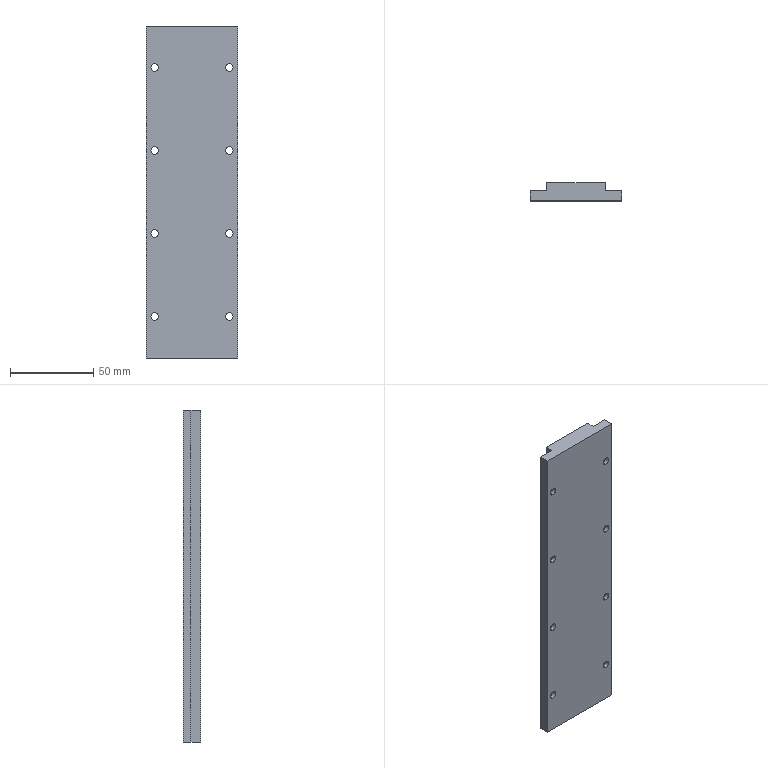Part | SolidWorks | features BaseBody 1 | 1 solid | 50 faces | box 55 x 10.7 x 200 mm | volume 97550 mm3 | cylinder 32 | plane 18 | commonest cylinder face diameters 4.5 x16 8 x16
STEP:
#1=CARTESIAN_POINT('',(5.,0.,27.25));
#2=VERTEX_POINT('',#1);
#3=CARTESIAN_POINT('',(5.,0.,22.75));
#4=VERTEX_POINT('',#3);
#5=CARTESIAN_POINT('',(5.,0.,25.));
#6=DIRECTION('',(0.,-1.,0.));
#7=DIRECTION('',(0.,0.,1.));
#8=AXIS2_PLACEMENT_3D('',#5,#6,#7);
#9=CIRCLE('',#8,2.25);
#10=EDGE_CURVE('',#2,#4,#9,.T.);
#11=ORIENTED_EDGE('',*,*,#10,.T.);
#12=CARTESIAN_POINT('',(5.,2.5,22.75));
#13=VERTEX_POINT('',#12);
#14=CARTESIAN_POINT('',(5.,6.,22.75));
#15=DIRECTION('',(0.,1.,0.));
#16=VECTOR('',#15,1000.);
#17=LINE('',#14,#16);
#18=EDGE_CURVE('',#4,#13,#17,.T.);
#19=ORIENTED_EDGE('',*,*,#18,.T.);
#20=CARTESIAN_POINT('',(5.,2.5,27.25));
#21=VERTEX_POINT('',#20);
#22=CARTESIAN_POINT('',(5.,2.5,25.));
#23=DIRECTION('',(0.,-1.,0.));
#24=DIRECTION('',(0.,0.,1.));
#25=AXIS2_PLACEMENT_3D('',#22,#23,#24);
#26=CIRCLE('',#25,2.25);
#27=EDGE_CURVE('',#21,#13,#26,.T.);
#28=ORIENTED_EDGE('',*,*,#27,.F.);
#29=CARTESIAN_POINT('',(5.,6.,27.25));
#30=DIRECTION('',(0.,1.,0.));
#31=VECTOR('',#30,1000.);
#32=LINE('',#29,#31);
#33=EDGE_CURVE('',#2,#21,#32,.T.);
#34=ORIENTED_EDGE('',*,*,#33,.F.);
#35=EDGE_LOOP('',(#11,#19,#28,#34));
#36=FACE_OUTER_BOUND('',#35,.T.);
#37=CARTESIAN_POINT('',(5.,6.,25.));
#38=DIRECTION('',(0.,1.,0.));
#39=DIRECTION('',(0.,0.,1.));
#40=AXIS2_PLACEMENT_3D('',#37,#38,#39);
#41=CYLINDRICAL_SURFACE('',#40,2.25);
#42=ADVANCED_FACE('',(#36),#41,.F.);
#43=CARTESIAN_POINT('',(50.,0.,27.25));
#44=VERTEX_POINT('',#43);
#45=CARTESIAN_POINT('',(50.,0.,22.75));
#46=VERTEX_POINT('',#45);
#47=CARTESIAN_POINT('',(50.,0.,25.));
#48=DIRECTION('',(0.,-1.,0.));
#49=DIRECTION('',(0.,0.,1.));
#50=AXIS2_PLACEMENT_3D('',#47,#48,#49);
#51=CIRCLE('',#50,2.25);
#52=EDGE_CURVE('',#44,#46,#51,.T.);
#53=ORIENTED_EDGE('',*,*,#52,.T.);
#54=CARTESIAN_POINT('',(50.,2.5,22.75));
#55=VERTEX_POINT('',#54);
#56=CARTESIAN_POINT('',(50.,6.,22.75));
#57=DIRECTION('',(0.,1.,0.));
#58=VECTOR('',#57,1000.);
#59=LINE('',#56,#58);
#60=EDGE_CURVE('',#46,#55,#59,.T.);
#61=ORIENTED_EDGE('',*,*,#60,.T.);
#62=CARTESIAN_POINT('',(50.,2.5,27.25));
#63=VERTEX_POINT('',#62);
#64=CARTESIAN_POINT('',(50.,2.5,25.));
#65=DIRECTION('',(0.,-1.,0.));
#66=DIRECTION('',(0.,0.,1.));
#67=AXIS2_PLACEMENT_3D('',#64,#65,#66);
#68=CIRCLE('',#67,2.25);
#69=EDGE_CURVE('',#63,#55,#68,.T.);
#70=ORIENTED_EDGE('',*,*,#69,.F.);
#71=CARTESIAN_POINT('',(50.,6.,27.25));
#72=DIRECTION('',(0.,1.,0.));
#73=VECTOR('',#72,1000.);
#74=LINE('',#71,#73);
#75=EDGE_CURVE('',#44,#63,#74,.T.);
#76=ORIENTED_EDGE('',*,*,#75,.F.);
#77=EDGE_LOOP('',(#53,#61,#70,#76));
#78=FACE_OUTER_BOUND('',#77,.T.);
#79=CARTESIAN_POINT('',(50.,6.,25.));
#80=DIRECTION('',(0.,1.,0.));
#81=DIRECTION('',(0.,0.,1.));
#82=AXIS2_PLACEMENT_3D('',#79,#80,#81);
#83=CYLINDRICAL_SURFACE('',#82,2.25);
#84=ADVANCED_FACE('',(#78),#83,.F.);
#85=CARTESIAN_POINT('',(5.,0.,77.25));
#86=VERTEX_POINT('',#85);
#87=CARTESIAN_POINT('',(5.,0.,72.75));
#88=VERTEX_POINT('',#87);
#89=CARTESIAN_POINT('',(5.,0.,75.));
#90=DIRECTION('',(0.,-1.,0.));
#91=DIRECTION('',(0.,0.,1.));
#92=AXIS2_PLACEMENT_3D('',#89,#90,#91);
#93=CIRCLE('',#92,2.25);
#94=EDGE_CURVE('',#86,#88,#93,.T.);
#95=ORIENTED_EDGE('',*,*,#94,.T.);
#96=CARTESIAN_POINT('',(5.,2.5,72.75));
#97=VERTEX_POINT('',#96);
#98=CARTESIAN_POINT('',(5.,6.,72.75));
#99=DIRECTION('',(0.,1.,0.));
#100=VECTOR('',#99,1000.);
#101=LINE('',#98,#100);
#102=EDGE_CURVE('',#88,#97,#101,.T.);
#103=ORIENTED_EDGE('',*,*,#102,.T.);
#104=CARTESIAN_POINT('',(5.,2.5,77.25));
#105=VERTEX_POINT('',#104);
#106=CARTESIAN_POINT('',(5.,2.5,75.));
#107=DIRECTION('',(0.,-1.,0.));
#108=DIRECTION('',(0.,0.,1.));
#109=AXIS2_PLACEMENT_3D('',#106,#107,#108);
#110=CIRCLE('',#109,2.25);
#111=EDGE_CURVE('',#105,#97,#110,.T.);
#112=ORIENTED_EDGE('',*,*,#111,.F.);
#113=CARTESIAN_POINT('',(5.,6.,77.25));
#114=DIRECTION('',(0.,1.,0.));
#115=VECTOR('',#114,1000.);
#116=LINE('',#113,#115);
#117=EDGE_CURVE('',#86,#105,#116,.T.);
#118=ORIENTED_EDGE('',*,*,#117,.F.);
#119=EDGE_LOOP('',(#95,#103,#112,#118));
#120=FACE_OUTER_BOUND('',#119,.T.);
#121=CARTESIAN_POINT('',(5.,6.,75.));
#122=DIRECTION('',(0.,1.,0.));
#123=DIRECTION('',(0.,0.,1.));
#124=AXIS2_PLACEMENT_3D('',#121,#122,#123);
#125=CYLINDRICAL_SURFACE('',#124,2.25);
#126=ADVANCED_FACE('',(#120),#125,.F.);
#127=CARTESIAN_POINT('',(50.,0.,77.25));
#128=VERTEX_POINT('',#127);
#129=CARTESIAN_POINT('',(50.,0.,72.75));
#130=VERTEX_POINT('',#129);
#131=CARTESIAN_POINT('',(50.,0.,75.));
#132=DIRECTION('',(0.,-1.,0.));
#133=DIRECTION('',(0.,0.,1.));
#134=AXIS2_PLACEMENT_3D('',#131,#132,#133);
#135=CIRCLE('',#134,2.25);
#136=EDGE_CURVE('',#128,#130,#135,.T.);
#137=ORIENTED_EDGE('',*,*,#136,.T.);
#138=CARTESIAN_POINT('',(50.,2.5,72.75));
#139=VERTEX_POINT('',#138);
#140=CARTESIAN_POINT('',(50.,6.,72.75));
#141=DIRECTION('',(0.,1.,0.));
#142=VECTOR('',#141,1000.);
#143=LINE('',#140,#142);
#144=EDGE_CURVE('',#130,#139,#143,.T.);
#145=ORIENTED_EDGE('',*,*,#144,.T.);
#146=CARTESIAN_POINT('',(50.,2.5,77.25));
#147=VERTEX_POINT('',#146);
#148=CARTESIAN_POINT('',(50.,2.5,75.));
#149=DIRECTION('',(0.,-1.,0.));
#150=DIRECTION('',(0.,0.,1.));
#151=AXIS2_PLACEMENT_3D('',#148,#149,#150);
#152=CIRCLE('',#151,2.25);
#153=EDGE_CURVE('',#147,#139,#152,.T.);
#154=ORIENTED_EDGE('',*,*,#153,.F.);
#155=CARTESIAN_POINT('',(50.,6.,77.25));
#156=DIRECTION('',(0.,1.,0.));
#157=VECTOR('',#156,1000.);
#158=LINE('',#155,#157);
#159=EDGE_CURVE('',#128,#147,#158,.T.);
#160=ORIENTED_EDGE('',*,*,#159,.F.);
#161=EDGE_LOOP('',(#137,#145,#154,#160));
#162=FACE_OUTER_BOUND('',#161,.T.);
#163=CARTESIAN_POINT('',(50.,6.,75.));
#164=DIRECTION('',(0.,1.,0.));
#165=DIRECTION('',(0.,0.,1.));
#166=AXIS2_PLACEMENT_3D('',#163,#164,#165);
#167=CYLINDRICAL_SURFACE('',#166,2.25);
#168=ADVANCED_FACE('',(#162),#167,.F.);
#169=CARTESIAN_POINT('',(5.,0.,127.25));
#170=VERTEX_POINT('',#169);
#171=CARTESIAN_POINT('',(5.,0.,122.75));
#172=VERTEX_POINT('',#171);
#173=CARTESIAN_POINT('',(5.,0.,125.));
#174=DIRECTION('',(0.,-1.,0.));
#175=DIRECTION('',(0.,0.,1.));
#176=AXIS2_PLACEMENT_3D('',#173,#174,#175);
#177=CIRCLE('',#176,2.25);
#178=EDGE_CURVE('',#170,#172,#177,.T.);
#179=ORIENTED_EDGE('',*,*,#178,.T.);
#180=CARTESIAN_POINT('',(5.,2.5,122.75));
#181=VERTEX_POINT('',#180);
#182=CARTESIAN_POINT('',(5.,6.,122.75));
#183=DIRECTION('',(0.,1.,0.));
#184=VECTOR('',#183,1000.);
#185=LINE('',#182,#184);
#186=EDGE_CURVE('',#172,#181,#185,.T.);
#187=ORIENTED_EDGE('',*,*,#186,.T.);
#188=CARTESIAN_POINT('',(5.,2.5,127.25));
#189=VERTEX_POINT('',#188);
#190=CARTESIAN_POINT('',(5.,2.5,125.));
#191=DIRECTION('',(0.,-1.,0.));
#192=DIRECTION('',(0.,0.,1.));
#193=AXIS2_PLACEMENT_3D('',#190,#191,#192);
#194=CIRCLE('',#193,2.25);
#195=EDGE_CURVE('',#189,#181,#194,.T.);
#196=ORIENTED_EDGE('',*,*,#195,.F.);
#197=CARTESIAN_POINT('',(5.,6.,127.25));
#198=DIRECTION('',(0.,1.,0.));
#199=VECTOR('',#198,1000.);
#200=LINE('',#197,#199);
#201=EDGE_CURVE('',#170,#189,#200,.T.);
#202=ORIENTED_EDGE('',*,*,#201,.F.);
#203=EDGE_LOOP('',(#179,#187,#196,#202));
#204=FACE_OUTER_BOUND('',#203,.T.);
#205=CARTESIAN_POINT('',(5.,6.,125.));
#206=DIRECTION('',(0.,1.,0.));
#207=DIRECTION('',(0.,0.,1.));
#208=AXIS2_PLACEMENT_3D('',#205,#206,#207);
#209=CYLINDRICAL_SURFACE('',#208,2.25);
#210=ADVANCED_FACE('',(#204),#209,.F.);
#211=CARTESIAN_POINT('',(50.,0.,127.25));
#212=VERTEX_POINT('',#211);
#213=CARTESIAN_POINT('',(50.,0.,122.75));
#214=VERTEX_POINT('',#213);
#215=CARTESIAN_POINT('',(50.,0.,125.));
#216=DIRECTION('',(0.,-1.,0.));
#217=DIRECTION('',(0.,0.,1.));
#218=AXIS2_PLACEMENT_3D('',#215,#216,#217);
#219=CIRCLE('',#218,2.25);
#220=EDGE_CURVE('',#212,#214,#219,.T.);
#221=ORIENTED_EDGE('',*,*,#220,.T.);
#222=CARTESIAN_POINT('',(50.,2.5,122.75));
#223=VERTEX_POINT('',#222);
#224=CARTESIAN_POINT('',(50.,6.,122.75));
#225=DIRECTION('',(0.,1.,0.));
#226=VECTOR('',#225,1000.);
#227=LINE('',#224,#226);
#228=EDGE_CURVE('',#214,#223,#227,.T.);
#229=ORIENTED_EDGE('',*,*,#228,.T.);
#230=CARTESIAN_POINT('',(50.,2.5,127.25));
#231=VERTEX_POINT('',#230);
#232=CARTESIAN_POINT('',(50.,2.5,125.));
#233=DIRECTION('',(0.,-1.,0.));
#234=DIRECTION('',(0.,0.,1.));
#235=AXIS2_PLACEMENT_3D('',#232,#233,#234);
#236=CIRCLE('',#235,2.25);
#237=EDGE_CURVE('',#231,#223,#236,.T.);
#238=ORIENTED_EDGE('',*,*,#237,.F.);
#239=CARTESIAN_POINT('',(50.,6.,127.25));
#240=DIRECTION('',(0.,1.,0.));
#241=VECTOR('',#240,1000.);
#242=LINE('',#239,#241);
#243=EDGE_CURVE('',#212,#231,#242,.T.);
#244=ORIENTED_EDGE('',*,*,#243,.F.);
#245=EDGE_LOOP('',(#221,#229,#238,#244));
#246=FACE_OUTER_BOUND('',#245,.T.);
#247=CARTESIAN_POINT('',(50.,6.,125.));
#248=DIRECTION('',(0.,1.,0.));
#249=DIRECTION('',(0.,0.,1.));
#250=AXIS2_PLACEMENT_3D('',#247,#248,#249);
#251=CYLINDRICAL_SURFACE('',#250,2.25);
#252=ADVANCED_FACE('',(#246),#251,.F.);
#253=CARTESIAN_POINT('',(5.,0.,177.25));
#254=VERTEX_POINT('',#253);
#255=CARTESIAN_POINT('',(5.,0.,172.75));
#256=VERTEX_POINT('',#255);
#257=CARTESIAN_POINT('',(5.,0.,175.));
#258=DIRECTION('',(0.,-1.,0.));
#259=DIRECTION('',(0.,0.,1.));
#260=AXIS2_PLACEMENT_3D('',#257,#258,#259);
#261=CIRCLE('',#260,2.25);
#262=EDGE_CURVE('',#254,#256,#261,.T.);
#263=ORIENTED_EDGE('',*,*,#262,.T.);
#264=CARTESIAN_POINT('',(5.,2.5,172.75));
#265=VERTEX_POINT('',#264);
#266=CARTESIAN_POINT('',(5.,6.,172.75));
#267=DIRECTION('',(0.,1.,0.));
#268=VECTOR('',#267,1000.);
#269=LINE('',#266,#268);
#270=EDGE_CURVE('',#256,#265,#269,.T.);
#271=ORIENTED_EDGE('',*,*,#270,.T.);
#272=CARTESIAN_POINT('',(5.,2.5,177.25));
#273=VERTEX_POINT('',#272);
#274=CARTESIAN_POINT('',(5.,2.5,175.));
#275=DIRECTION('',(0.,-1.,0.));
#276=DIRECTION('',(0.,0.,1.));
#277=AXIS2_PLACEMENT_3D('',#274,#275,#276);
#278=CIRCLE('',#277,2.25);
#279=EDGE_CURVE('',#273,#265,#278,.T.);
#280=ORIENTED_EDGE('',*,*,#279,.F.);
#281=CARTESIAN_POINT('',(5.,6.,177.25));
#282=DIRECTION('',(0.,1.,0.));
#283=VECTOR('',#282,1000.);
#284=LINE('',#281,#283);
#285=EDGE_CURVE('',#254,#273,#284,.T.);
#286=ORIENTED_EDGE('',*,*,#285,.F.);
#287=EDGE_LOOP('',(#263,#271,#280,#286));
#288=FACE_OUTER_BOUND('',#287,.T.);
#289=CARTESIAN_POINT('',(5.,6.,175.));
#290=DIRECTION('',(0.,1.,0.));
#291=DIRECTION('',(0.,0.,1.));
#292=AXIS2_PLACEMENT_3D('',#289,#290,#291);
#293=CYLINDRICAL_SURFACE('',#292,2.25);
#294=ADVANCED_FACE('',(#288),#293,.F.);
#295=CARTESIAN_POINT('',(50.,0.,177.25));
#296=VERTEX_POINT('',#295);
#297=CARTESIAN_POINT('',(50.,0.,172.75));
#298=VERTEX_POINT('',#297);
#299=CARTESIAN_POINT('',(50.,0.,175.));
#300=DIRECTION('',(0.,-1.,0.));
#301=DIRECTION('',(0.,0.,1.));
#302=AXIS2_PLACEMENT_3D('',#299,#300,#301);
#303=CIRCLE('',#302,2.25);
#304=EDGE_CURVE('',#296,#298,#303,.T.);
#305=ORIENTED_EDGE('',*,*,#304,.T.);
#306=CARTESIAN_POINT('',(50.,2.5,172.75));
#307=VERTEX_POINT('',#306);
#308=CARTESIAN_POINT('',(50.,6.,172.75));
#309=DIRECTION('',(0.,1.,0.));
#310=VECTOR('',#309,1000.);
#311=LINE('',#308,#310);
#312=EDGE_CURVE('',#298,#307,#311,.T.);
#313=ORIENTED_EDGE('',*,*,#312,.T.);
#314=CARTESIAN_POINT('',(50.,2.5,177.25));
#315=VERTEX_POINT('',#314);
#316=CARTESIAN_POINT('',(50.,2.5,175.));
#317=DIRECTION('',(0.,-1.,0.));
#318=DIRECTION('',(0.,0.,1.));
#319=AXIS2_PLACEMENT_3D('',#316,#317,#318);
#320=CIRCLE('',#319,2.25);
#321=EDGE_CURVE('',#315,#307,#320,.T.);
#322=ORIENTED_EDGE('',*,*,#321,.F.);
#323=CARTESIAN_POINT('',(50.,6.,177.25));
#324=DIRECTION('',(0.,1.,0.));
#325=VECTOR('',#324,1000.);
#326=LINE('',#323,#325);
#327=EDGE_CURVE('',#296,#315,#326,.T.);
#328=ORIENTED_EDGE('',*,*,#327,.F.);
#329=EDGE_LOOP('',(#305,#313,#322,#328));
#330=FACE_OUTER_BOUND('',#329,.T.);
#331=CARTESIAN_POINT('',(50.,6.,175.));
#332=DIRECTION('',(0.,1.,0.));
#333=DIRECTION('',(0.,0.,1.));
#334=AXIS2_PLACEMENT_3D('',#331,#332,#333);
#335=CYLINDRICAL_SURFACE('',#334,2.25);
#336=ADVANCED_FACE('',(#330),#335,.F.);
#337=CARTESIAN_POINT('',(5.,2.5,29.));
#338=VERTEX_POINT('',#337);
#339=CARTESIAN_POINT('',(5.,2.5,21.));
#340=VERTEX_POINT('',#339);
#341=CARTESIAN_POINT('',(5.,2.5,25.));
#342=DIRECTION('',(0.,-1.,0.));
#343=DIRECTION('',(0.,0.,1.));
#344=AXIS2_PLACEMENT_3D('',#341,#342,#343);
#345=CIRCLE('',#344,4.);
#346=EDGE_CURVE('',#338,#340,#345,.T.);
#347=ORIENTED_EDGE('',*,*,#346,.T.);
#348=CARTESIAN_POINT('',(5.,6.,21.));
#349=VERTEX_POINT('',#348);
#350=CARTESIAN_POINT('',(5.,6.,21.));
#351=DIRECTION('',(0.,1.,0.));
#352=VECTOR('',#351,1000.);
#353=LINE('',#350,#352);
#354=EDGE_CURVE('',#340,#349,#353,.T.);
#355=ORIENTED_EDGE('',*,*,#354,.T.);
#356=CARTESIAN_POINT('',(5.,6.,29.));
#357=VERTEX_POINT('',#356);
#358=CARTESIAN_POINT('',(5.,6.,25.));
#359=DIRECTION('',(0.,-1.,0.));
#360=DIRECTION('',(0.,0.,1.));
#361=AXIS2_PLACEMENT_3D('',#358,#359,#360);
#362=CIRCLE('',#361,4.);
#363=EDGE_CURVE('',#357,#349,#362,.T.);
#364=ORIENTED_EDGE('',*,*,#363,.F.);
#365=CARTESIAN_POINT('',(5.,6.,29.));
#366=DIRECTION('',(0.,1.,0.));
#367=VECTOR('',#366,1000.);
#368=LINE('',#365,#367);
#369=EDGE_CURVE('',#338,#357,#368,.T.);
#370=ORIENTED_EDGE('',*,*,#369,.F.);
#371=EDGE_LOOP('',(#347,#355,#364,#370));
#372=FACE_OUTER_BOUND('',#371,.T.);
#373=CARTESIAN_POINT('',(5.,6.,25.));
#374=DIRECTION('',(0.,1.,0.));
#375=DIRECTION('',(0.,0.,1.));
#376=AXIS2_PLACEMENT_3D('',#373,#374,#375);
#377=CYLINDRICAL_SURFACE('',#376,4.);
#378=ADVANCED_FACE('',(#372),#377,.F.);
#379=CARTESIAN_POINT('',(5.,2.5,79.));
#380=VERTEX_POINT('',#379);
#381=CARTESIAN_POINT('',(5.,2.5,71.));
#382=VERTEX_POINT('',#381);
#383=CARTESIAN_POINT('',(5.,2.5,75.));
#384=DIRECTION('',(0.,-1.,0.));
#385=DIRECTION('',(0.,0.,1.));
#386=AXIS2_PLACEMENT_3D('',#383,#384,#385);
#387=CIRCLE('',#386,4.);
#388=EDGE_CURVE('',#380,#382,#387,.T.);
#389=ORIENTED_EDGE('',*,*,#388,.T.);
#390=CARTESIAN_POINT('',(5.,6.,71.));
#391=VERTEX_POINT('',#390);
#392=CARTESIAN_POINT('',(5.,6.,71.));
#393=DIRECTION('',(0.,1.,0.));
#394=VECTOR('',#393,1000.);
#395=LINE('',#392,#394);
#396=EDGE_CURVE('',#382,#391,#395,.T.);
#397=ORIENTED_EDGE('',*,*,#396,.T.);
#398=CARTESIAN_POINT('',(5.,6.,79.));
#399=VERTEX_POINT('',#398);
#400=CARTESIAN_POINT('',(5.,6.,75.));
#401=DIRECTION('',(0.,-1.,0.));
#402=DIRECTION('',(0.,0.,1.));
#403=AXIS2_PLACEMENT_3D('',#400,#401,#402);
#404=CIRCLE('',#403,4.);
#405=EDGE_CURVE('',#399,#391,#404,.T.);
#406=ORIENTED_EDGE('',*,*,#405,.F.);
#407=CARTESIAN_POINT('',(5.,6.,79.));
#408=DIRECTION('',(0.,1.,0.));
#409=VECTOR('',#408,1000.);
#410=LINE('',#407,#409);
#411=EDGE_CURVE('',#380,#399,#410,.T.);
#412=ORIENTED_EDGE('',*,*,#411,.F.);
#413=EDGE_LOOP('',(#389,#397,#406,#412));
#414=FACE_OUTER_BOUND('',#413,.T.);
#415=CARTESIAN_POINT('',(5.,6.,75.));
#416=DIRECTION('',(0.,1.,0.));
#417=DIRECTION('',(0.,0.,1.));
#418=AXIS2_PLACEMENT_3D('',#415,#416,#417);
#419=CYLINDRICAL_SURFACE('',#418,4.);
#420=ADVANCED_FACE('',(#414),#419,.F.);
#421=CARTESIAN_POINT('',(5.,2.5,129.));
#422=VERTEX_POINT('',#421);
#423=CARTESIAN_POINT('',(5.,2.5,121.));
#424=VERTEX_POINT('',#423);
#425=CARTESIAN_POINT('',(5.,2.5,125.));
#426=DIRECTION('',(0.,-1.,0.));
#427=DIRECTION('',(0.,0.,1.));
#428=AXIS2_PLACEMENT_3D('',#425,#426,#427);
#429=CIRCLE('',#428,4.);
#430=EDGE_CURVE('',#422,#424,#429,.T.);
#431=ORIENTED_EDGE('',*,*,#430,.T.);
#432=CARTESIAN_POINT('',(5.,6.,121.));
#433=VERTEX_POINT('',#432);
#434=CARTESIAN_POINT('',(5.,6.,121.));
#435=DIRECTION('',(0.,1.,0.));
#436=VECTOR('',#435,1000.);
#437=LINE('',#434,#436);
#438=EDGE_CURVE('',#424,#433,#437,.T.);
#439=ORIENTED_EDGE('',*,*,#438,.T.);
#440=CARTESIAN_POINT('',(5.,6.,129.));
#441=VERTEX_POINT('',#440);
#442=CARTESIAN_POINT('',(5.,6.,125.));
#443=DIRECTION('',(0.,-1.,0.));
#444=DIRECTION('',(0.,0.,1.));
#445=AXIS2_PLACEMENT_3D('',#442,#443,#444);
#446=CIRCLE('',#445,4.);
#447=EDGE_CURVE('',#441,#433,#446,.T.);
#448=ORIENTED_EDGE('',*,*,#447,.F.);
#449=CARTESIAN_POINT('',(5.,6.,129.));
#450=DIRECTION('',(0.,1.,0.));
#451=VECTOR('',#450,1000.);
#452=LINE('',#449,#451);
#453=EDGE_CURVE('',#422,#441,#452,.T.);
#454=ORIENTED_EDGE('',*,*,#453,.F.);
#455=EDGE_LOOP('',(#431,#439,#448,#454));
#456=FACE_OUTER_BOUND('',#455,.T.);
#457=CARTESIAN_POINT('',(5.,6.,125.));
#458=DIRECTION('',(0.,1.,0.));
#459=DIRECTION('',(0.,0.,1.));
#460=AXIS2_PLACEMENT_3D('',#457,#458,#459);
#461=CYLINDRICAL_SURFACE('',#460,4.);
#462=ADVANCED_FACE('',(#456),#461,.F.);
#463=CARTESIAN_POINT('',(5.,2.5,179.));
#464=VERTEX_POINT('',#463);
#465=CARTESIAN_POINT('',(5.,2.5,171.));
#466=VERTEX_POINT('',#465);
#467=CARTESIAN_POINT('',(5.,2.5,175.));
#468=DIRECTION('',(0.,-1.,0.));
#469=DIRECTION('',(0.,0.,1.));
#470=AXIS2_PLACEMENT_3D('',#467,#468,#469);
#471=CIRCLE('',#470,4.);
#472=EDGE_CURVE('',#464,#466,#471,.T.);
#473=ORIENTED_EDGE('',*,*,#472,.T.);
#474=CARTESIAN_POINT('',(5.,6.,171.));
#475=VERTEX_POINT('',#474);
#476=CARTESIAN_POINT('',(5.,6.,171.));
#477=DIRECTION('',(0.,1.,0.));
#478=VECTOR('',#477,1000.);
#479=LINE('',#476,#478);
#480=EDGE_CURVE('',#466,#475,#479,.T.);
#481=ORIENTED_EDGE('',*,*,#480,.T.);
#482=CARTESIAN_POINT('',(5.,6.,179.));
#483=VERTEX_POINT('',#482);
#484=CARTESIAN_POINT('',(5.,6.,175.));
#485=DIRECTION('',(0.,-1.,0.));
#486=DIRECTION('',(0.,0.,1.));
#487=AXIS2_PLACEMENT_3D('',#484,#485,#486);
#488=CIRCLE('',#487,4.);
#489=EDGE_CURVE('',#483,#475,#488,.T.);
#490=ORIENTED_EDGE('',*,*,#489,.F.);
#491=CARTESIAN_POINT('',(5.,6.,179.));
#492=DIRECTION('',(0.,1.,0.));
#493=VECTOR('',#492,1000.);
#494=LINE('',#491,#493);
#495=EDGE_CURVE('',#464,#483,#494,.T.);
#496=ORIENTED_EDGE('',*,*,#495,.F.);
#497=EDGE_LOOP('',(#473,#481,#490,#496));
#498=FACE_OUTER_BOUND('',#497,.T.);
#499=CARTESIAN_POINT('',(5.,6.,175.));
#500=DIRECTION('',(0.,1.,0.));
#501=DIRECTION('',(0.,0.,1.));
#502=AXIS2_PLACEMENT_3D('',#499,#500,#501);
#503=CYLINDRICAL_SURFACE('',#502,4.);
#504=ADVANCED_FACE('',(#498),#503,.F.);
#505=CARTESIAN_POINT('',(50.,2.5,29.));
#506=VERTEX_POINT('',#505);
#507=CARTESIAN_POINT('',(50.,2.5,21.));
#508=VERTEX_POINT('',#507);
#509=CARTESIAN_POINT('',(50.,2.5,25.));
#510=DIRECTION('',(0.,-1.,0.));
#511=DIRECTION('',(0.,0.,1.));
#512=AXIS2_PLACEMENT_3D('',#509,#510,#511);
#513=CIRCLE('',#512,4.);
#514=EDGE_CURVE('',#506,#508,#513,.T.);
#515=ORIENTED_EDGE('',*,*,#514,.T.);
#516=CARTESIAN_POINT('',(50.,6.,21.));
#517=VERTEX_POINT('',#516);
#518=CARTESIAN_POINT('',(50.,6.,21.));
#519=DIRECTION('',(0.,1.,0.));
#520=VECTOR('',#519,1000.);
#521=LINE('',#518,#520);
#522=EDGE_CURVE('',#508,#517,#521,.T.);
#523=ORIENTED_EDGE('',*,*,#522,.T.);
#524=CARTESIAN_POINT('',(50.,6.,29.));
#525=VERTEX_POINT('',#524);
#526=CARTESIAN_POINT('',(50.,6.,25.));
#527=DIRECTION('',(0.,-1.,0.));
#528=DIRECTION('',(0.,0.,1.));
#529=AXIS2_PLACEMENT_3D('',#526,#527,#528);
#530=CIRCLE('',#529,4.);
#531=EDGE_CURVE('',#525,#517,#530,.T.);
#532=ORIENTED_EDGE('',*,*,#531,.F.);
#533=CARTESIAN_POINT('',(50.,6.,29.));
#534=DIRECTION('',(0.,1.,0.));
#535=VECTOR('',#534,1000.);
#536=LINE('',#533,#535);
#537=EDGE_CURVE('',#506,#525,#536,.T.);
#538=ORIENTED_EDGE('',*,*,#537,.F.);
#539=EDGE_LOOP('',(#515,#523,#532,#538));
#540=FACE_OUTER_BOUND('',#539,.T.);
#541=CARTESIAN_POINT('',(50.,6.,25.));
#542=DIRECTION('',(0.,1.,0.));
#543=DIRECTION('',(0.,0.,1.));
#544=AXIS2_PLACEMENT_3D('',#541,#542,#543);
#545=CYLINDRICAL_SURFACE('',#544,4.);
#546=ADVANCED_FACE('',(#540),#545,.F.);
#547=CARTESIAN_POINT('',(50.,2.5,79.));
#548=VERTEX_POINT('',#547);
#549=CARTESIAN_POINT('',(50.,2.5,71.));
#550=VERTEX_POINT('',#549);
#551=CARTESIAN_POINT('',(50.,2.5,75.));
#552=DIRECTION('',(0.,-1.,0.));
#553=DIRECTION('',(0.,0.,1.));
#554=AXIS2_PLACEMENT_3D('',#551,#552,#553);
#555=CIRCLE('',#554,4.);
#556=EDGE_CURVE('',#548,#550,#555,.T.);
#557=ORIENTED_EDGE('',*,*,#556,.T.);
#558=CARTESIAN_POINT('',(50.,6.,71.));
#559=VERTEX_POINT('',#558);
#560=CARTESIAN_POINT('',(50.,6.,71.));
#561=DIRECTION('',(0.,1.,0.));
#562=VECTOR('',#561,1000.);
#563=LINE('',#560,#562);
#564=EDGE_CURVE('',#550,#559,#563,.T.);
#565=ORIENTED_EDGE('',*,*,#564,.T.);
#566=CARTESIAN_POINT('',(50.,6.,79.));
#567=VERTEX_POINT('',#566);
#568=CARTESIAN_POINT('',(50.,6.,75.));
#569=DIRECTION('',(0.,-1.,0.));
#570=DIRECTION('',(0.,0.,1.));
#571=AXIS2_PLACEMENT_3D('',#568,#569,#570);
#572=CIRCLE('',#571,4.);
#573=EDGE_CURVE('',#567,#559,#572,.T.);
#574=ORIENTED_EDGE('',*,*,#573,.F.);
#575=CARTESIAN_POINT('',(50.,6.,79.));
#576=DIRECTION('',(0.,1.,0.));
#577=VECTOR('',#576,1000.);
#578=LINE('',#575,#577);
#579=EDGE_CURVE('',#548,#567,#578,.T.);
#580=ORIENTED_EDGE('',*,*,#579,.F.);
#581=EDGE_LOOP('',(#557,#565,#574,#580));
#582=FACE_OUTER_BOUND('',#581,.T.);
#583=CARTESIAN_POINT('',(50.,6.,75.));
#584=DIRECTION('',(0.,1.,0.));
#585=DIRECTION('',(0.,0.,1.));
#586=AXIS2_PLACEMENT_3D('',#583,#584,#585);
#587=CYLINDRICAL_SURFACE('',#586,4.);
#588=ADVANCED_FACE('',(#582),#587,.F.);
#589=CARTESIAN_POINT('',(50.,2.5,129.));
#590=VERTEX_POINT('',#589);
#591=CARTESIAN_POINT('',(50.,2.5,121.));
#592=VERTEX_POINT('',#591);
#593=CARTESIAN_POINT('',(50.,2.5,125.));
#594=DIRECTION('',(0.,-1.,0.));
#595=DIRECTION('',(0.,0.,1.));
#596=AXIS2_PLACEMENT_3D('',#593,#594,#595);
#597=CIRCLE('',#596,4.);
#598=EDGE_CURVE('',#590,#592,#597,.T.);
#599=ORIENTED_EDGE('',*,*,#598,.T.);
#600=CARTESIAN_POINT('',(50.,6.,121.));
#601=VERTEX_POINT('',#600);
#602=CARTESIAN_POINT('',(50.,6.,121.));
#603=DIRECTION('',(0.,1.,0.));
#604=VECTOR('',#603,1000.);
#605=LINE('',#602,#604);
#606=EDGE_CURVE('',#592,#601,#605,.T.);
#607=ORIENTED_EDGE('',*,*,#606,.T.);
#608=CARTESIAN_POINT('',(50.,6.,129.));
#609=VERTEX_POINT('',#608);
#610=CARTESIAN_POINT('',(50.,6.,125.));
#611=DIRECTION('',(0.,-1.,0.));
#612=DIRECTION('',(0.,0.,1.));
#613=AXIS2_PLACEMENT_3D('',#610,#611,#612);
#614=CIRCLE('',#613,4.);
#615=EDGE_CURVE('',#609,#601,#614,.T.);
#616=ORIENTED_EDGE('',*,*,#615,.F.);
#617=CARTESIAN_POINT('',(50.,6.,129.));
#618=DIRECTION('',(0.,1.,0.));
#619=VECTOR('',#618,1000.);
#620=LINE('',#617,#619);
#621=EDGE_CURVE('',#590,#609,#620,.T.);
#622=ORIENTED_EDGE('',*,*,#621,.F.);
#623=EDGE_LOOP('',(#599,#607,#616,#622));
#624=FACE_OUTER_BOUND('',#623,.T.);
#625=CARTESIAN_POINT('',(50.,6.,125.));
#626=DIRECTION('',(0.,1.,0.));
#627=DIRECTION('',(0.,0.,1.));
#628=AXIS2_PLACEMENT_3D('',#625,#626,#627);
#629=CYLINDRICAL_SURFACE('',#628,4.);
#630=ADVANCED_FACE('',(#624),#629,.F.);
#631=CARTESIAN_POINT('',(50.,2.5,179.));
#632=VERTEX_POINT('',#631);
#633=CARTESIAN_POINT('',(50.,2.5,171.));
#634=VERTEX_POINT('',#633);
#635=CARTESIAN_POINT('',(50.,2.5,175.));
#636=DIRECTION('',(0.,-1.,0.));
#637=DIRECTION('',(0.,0.,1.));
#638=AXIS2_PLACEMENT_3D('',#635,#636,#637);
#639=CIRCLE('',#638,4.);
#640=EDGE_CURVE('',#632,#634,#639,.T.);
#641=ORIENTED_EDGE('',*,*,#640,.T.);
#642=CARTESIAN_POINT('',(50.,6.,171.));
#643=VERTEX_POINT('',#642);
#644=CARTESIAN_POINT('',(50.,6.,171.));
#645=DIRECTION('',(0.,1.,0.));
#646=VECTOR('',#645,1000.);
#647=LINE('',#644,#646);
#648=EDGE_CURVE('',#634,#643,#647,.T.);
#649=ORIENTED_EDGE('',*,*,#648,.T.);
#650=CARTESIAN_POINT('',(50.,6.,179.));
#651=VERTEX_POINT('',#650);
#652=CARTESIAN_POINT('',(50.,6.,175.));
#653=DIRECTION('',(0.,-1.,0.));
#654=DIRECTION('',(0.,0.,1.));
#655=AXIS2_PLACEMENT_3D('',#652,#653,#654);
#656=CIRCLE('',#655,4.);
#657=EDGE_CURVE('',#651,#643,#656,.T.);
#658=ORIENTED_EDGE('',*,*,#657,.F.);
#659=CARTESIAN_POINT('',(50.,6.,179.));
#660=DIRECTION('',(0.,1.,0.));
#661=VECTOR('',#660,1000.);
#662=LINE('',#659,#661);
#663=EDGE_CURVE('',#632,#651,#662,.T.);
#664=ORIENTED_EDGE('',*,*,#663,.F.);
#665=EDGE_LOOP('',(#641,#649,#658,#664));
#666=FACE_OUTER_BOUND('',#665,.T.);
#667=CARTESIAN_POINT('',(50.,6.,175.));
#668=DIRECTION('',(0.,1.,0.));
#669=DIRECTION('',(0.,0.,1.));
#670=AXIS2_PLACEMENT_3D('',#667,#668,#669);
#671=CYLINDRICAL_SURFACE('',#670,4.);
#672=ADVANCED_FACE('',(#666),#671,.F.);
#673=CARTESIAN_POINT('',(55.,0.,200.));
#674=VERTEX_POINT('',#673);
#675=CARTESIAN_POINT('',(55.,0.,0.));
#676=VERTEX_POINT('',#675);
#677=CARTESIAN_POINT('',(55.,0.,200.));
#678=DIRECTION('',(0.,0.,-1.));
#679=VECTOR('',#678,1000.);
#680=LINE('',#677,#679);
#681=EDGE_CURVE('',#674,#676,#680,.T.);
#682=ORIENTED_EDGE('',*,*,#681,.F.);
#683=CARTESIAN_POINT('',(0.,0.,200.));
#684=VERTEX_POINT('',#683);
#685=CARTESIAN_POINT('',(0.,0.,200.));
#686=DIRECTION('',(1.,0.,0.));
#687=VECTOR('',#686,1000.);
#688=LINE('',#685,#687);
#689=EDGE_CURVE('',#684,#674,#688,.T.);
#690=ORIENTED_EDGE('',*,*,#689,.F.);
#691=CARTESIAN_POINT('',(0.,0.,0.));
#692=VERTEX_POINT('',#691);
#693=CARTESIAN_POINT('',(0.,0.,200.));
#694=DIRECTION('',(0.,0.,1.));
#695=VECTOR('',#694,1000.);
#696=LINE('',#693,#695);
#697=EDGE_CURVE('',#692,#684,#696,.T.);
#698=ORIENTED_EDGE('',*,*,#697,.F.);
#699=CARTESIAN_POINT('',(0.,0.,0.));
#700=DIRECTION('',(-1.,0.,0.));
#701=VECTOR('',#700,1000.);
#702=LINE('',#699,#701);
#703=EDGE_CURVE('',#676,#692,#702,.T.);
#704=ORIENTED_EDGE('',*,*,#703,.F.);
#705=EDGE_LOOP('',(#682,#690,#698,#704));
#706=FACE_OUTER_BOUND('',#705,.T.);
#707=ORIENTED_EDGE('',*,*,#10,.F.);
#708=CARTESIAN_POINT('',(5.,0.,25.));
#709=DIRECTION('',(0.,-1.,0.));
#710=DIRECTION('',(0.,0.,1.));
#711=AXIS2_PLACEMENT_3D('',#708,#709,#710);
#712=CIRCLE('',#711,2.25);
#713=EDGE_CURVE('',#4,#2,#712,.T.);
#714=ORIENTED_EDGE('',*,*,#713,.F.);
#715=EDGE_LOOP('',(#707,#714));
#716=FACE_BOUND('',#715,.T.);
#717=ORIENTED_EDGE('',*,*,#52,.F.);
#718=CARTESIAN_POINT('',(50.,0.,25.));
#719=DIRECTION('',(0.,-1.,0.));
#720=DIRECTION('',(0.,0.,1.));
#721=AXIS2_PLACEMENT_3D('',#718,#719,#720);
#722=CIRCLE('',#721,2.25);
#723=EDGE_CURVE('',#46,#44,#722,.T.);
#724=ORIENTED_EDGE('',*,*,#723,.F.);
#725=EDGE_LOOP('',(#717,#724));
#726=FACE_BOUND('',#725,.T.);
#727=ORIENTED_EDGE('',*,*,#94,.F.);
#728=CARTESIAN_POINT('',(5.,0.,75.));
#729=DIRECTION('',(0.,-1.,0.));
#730=DIRECTION('',(0.,0.,1.));
#731=AXIS2_PLACEMENT_3D('',#728,#729,#730);
#732=CIRCLE('',#731,2.25);
#733=EDGE_CURVE('',#88,#86,#732,.T.);
#734=ORIENTED_EDGE('',*,*,#733,.F.);
#735=EDGE_LOOP('',(#727,#734));
#736=FACE_BOUND('',#735,.T.);
#737=ORIENTED_EDGE('',*,*,#136,.F.);
#738=CARTESIAN_POINT('',(50.,0.,75.));
#739=DIRECTION('',(0.,-1.,0.));
#740=DIRECTION('',(0.,0.,1.));
#741=AXIS2_PLACEMENT_3D('',#738,#739,#740);
#742=CIRCLE('',#741,2.25);
#743=EDGE_CURVE('',#130,#128,#742,.T.);
#744=ORIENTED_EDGE('',*,*,#743,.F.);
#745=EDGE_LOOP('',(#737,#744));
#746=FACE_BOUND('',#745,.T.);
#747=ORIENTED_EDGE('',*,*,#178,.F.);
#748=CARTESIAN_POINT('',(5.,0.,125.));
#749=DIRECTION('',(0.,-1.,0.));
#750=DIRECTION('',(0.,0.,1.));
#751=AXIS2_PLACEMENT_3D('',#748,#749,#750);
#752=CIRCLE('',#751,2.25);
#753=EDGE_CURVE('',#172,#170,#752,.T.);
#754=ORIENTED_EDGE('',*,*,#753,.F.);
#755=EDGE_LOOP('',(#747,#754));
#756=FACE_BOUND('',#755,.T.);
#757=ORIENTED_EDGE('',*,*,#220,.F.);
#758=CARTESIAN_POINT('',(50.,0.,125.));
#759=DIRECTION('',(0.,-1.,0.));
#760=DIRECTION('',(0.,0.,1.));
#761=AXIS2_PLACEMENT_3D('',#758,#759,#760);
#762=CIRCLE('',#761,2.25);
#763=EDGE_CURVE('',#214,#212,#762,.T.);
#764=ORIENTED_EDGE('',*,*,#763,.F.);
#765=EDGE_LOOP('',(#757,#764));
#766=FACE_BOUND('',#765,.T.);
#767=ORIENTED_EDGE('',*,*,#262,.F.);
#768=CARTESIAN_POINT('',(5.,0.,175.));
#769=DIRECTION('',(0.,-1.,0.));
#770=DIRECTION('',(0.,0.,1.));
#771=AXIS2_PLACEMENT_3D('',#768,#769,#770);
#772=CIRCLE('',#771,2.25);
#773=EDGE_CURVE('',#256,#254,#772,.T.);
#774=ORIENTED_EDGE('',*,*,#773,.F.);
#775=EDGE_LOOP('',(#767,#774));
#776=FACE_BOUND('',#775,.T.);
#777=ORIENTED_EDGE('',*,*,#304,.F.);
#778=CARTESIAN_POINT('',(50.,0.,175.));
#779=DIRECTION('',(0.,-1.,0.));
#780=DIRECTION('',(0.,0.,1.));
#781=AXIS2_PLACEMENT_3D('',#778,#779,#780);
#782=CIRCLE('',#781,2.25);
#783=EDGE_CURVE('',#298,#296,#782,.T.);
#784=ORIENTED_EDGE('',*,*,#783,.F.);
#785=EDGE_LOOP('',(#777,#784));
#786=FACE_BOUND('',#785,.T.);
#787=CARTESIAN_POINT('',(0.,0.,200.));
#788=DIRECTION('',(0.,1.,0.));
#789=DIRECTION('',(0.,0.,1.));
#790=AXIS2_PLACEMENT_3D('',#787,#788,#789);
#791=PLANE('',#790);
#792=ADVANCED_FACE('',(#706,#716,#726,#736,#746,#756,#766,#776,#786),#791,.F.);
#793=CARTESIAN_POINT('',(9.8,6.,0.));
#794=VERTEX_POINT('',#793);
#795=CARTESIAN_POINT('',(9.8,10.7,0.));
#796=VERTEX_POINT('',#795);
#797=CARTESIAN_POINT('',(9.8,0.,0.));
#798=DIRECTION('',(0.,1.,0.));
#799=VECTOR('',#798,1000.);
#800=LINE('',#797,#799);
#801=EDGE_CURVE('',#794,#796,#800,.T.);
#802=ORIENTED_EDGE('',*,*,#801,.T.);
#803=CARTESIAN_POINT('',(45.2,10.7,0.));
#804=VERTEX_POINT('',#803);
#805=CARTESIAN_POINT('',(0.,10.7,0.));
#806=DIRECTION('',(1.,0.,0.));
#807=VECTOR('',#806,1000.);
#808=LINE('',#805,#807);
#809=EDGE_CURVE('',#796,#804,#808,.T.);
#810=ORIENTED_EDGE('',*,*,#809,.T.);
#811=CARTESIAN_POINT('',(45.2,6.,0.));
#812=VERTEX_POINT('',#811);
#813=CARTESIAN_POINT('',(45.2,0.,0.));
#814=DIRECTION('',(0.,-1.,0.));
#815=VECTOR('',#814,1000.);
#816=LINE('',#813,#815);
#817=EDGE_CURVE('',#804,#812,#816,.T.);
#818=ORIENTED_EDGE('',*,*,#817,.T.);
#819=CARTESIAN_POINT('',(55.,6.,0.));
#820=VERTEX_POINT('',#819);
#821=CARTESIAN_POINT('',(0.,6.,0.));
#822=DIRECTION('',(1.,0.,0.));
#823=VECTOR('',#822,1000.);
#824=LINE('',#821,#823);
#825=EDGE_CURVE('',#812,#820,#824,.T.);
#826=ORIENTED_EDGE('',*,*,#825,.T.);
#827=CARTESIAN_POINT('',(55.,0.,0.));
#828=DIRECTION('',(0.,-1.,0.));
#829=VECTOR('',#828,1000.);
#830=LINE('',#827,#829);
#831=EDGE_CURVE('',#820,#676,#830,.T.);
#832=ORIENTED_EDGE('',*,*,#831,.T.);
#833=ORIENTED_EDGE('',*,*,#703,.T.);
#834=CARTESIAN_POINT('',(0.,6.,0.));
#835=VERTEX_POINT('',#834);
#836=CARTESIAN_POINT('',(0.,0.,0.));
#837=DIRECTION('',(0.,1.,0.));
#838=VECTOR('',#837,1000.);
#839=LINE('',#836,#838);
#840=EDGE_CURVE('',#692,#835,#839,.T.);
#841=ORIENTED_EDGE('',*,*,#840,.T.);
#842=CARTESIAN_POINT('',(0.,6.,0.));
#843=DIRECTION('',(1.,0.,0.));
#844=VECTOR('',#843,1000.);
#845=LINE('',#842,#844);
#846=EDGE_CURVE('',#835,#794,#845,.T.);
#847=ORIENTED_EDGE('',*,*,#846,.T.);
#848=EDGE_LOOP('',(#802,#810,#818,#826,#832,#833,#841,#847));
#849=FACE_OUTER_BOUND('',#848,.T.);
#850=CARTESIAN_POINT('',(0.,0.,0.));
#851=DIRECTION('',(0.,0.,-1.));
#852=DIRECTION('',(-1.,0.,0.));
#853=AXIS2_PLACEMENT_3D('',#850,#851,#852);
#854=PLANE('',#853);
#855=ADVANCED_FACE('',(#849),#854,.T.);
#856=CARTESIAN_POINT('',(55.,6.,200.));
#857=VERTEX_POINT('',#856);
#858=CARTESIAN_POINT('',(55.,6.,200.));
#859=DIRECTION('',(0.,0.,-1.));
#860=VECTOR('',#859,1000.);
#861=LINE('',#858,#860);
#862=EDGE_CURVE('',#857,#820,#861,.T.);
#863=ORIENTED_EDGE('',*,*,#862,.F.);
#864=CARTESIAN_POINT('',(55.,0.,200.));
#865=DIRECTION('',(0.,1.,0.));
#866=VECTOR('',#865,1000.);
#867=LINE('',#864,#866);
#868=EDGE_CURVE('',#674,#857,#867,.T.);
#869=ORIENTED_EDGE('',*,*,#868,.F.);
#870=ORIENTED_EDGE('',*,*,#681,.T.);
#871=ORIENTED_EDGE('',*,*,#831,.F.);
#872=EDGE_LOOP('',(#863,#869,#870,#871));
#873=FACE_OUTER_BOUND('',#872,.T.);
#874=CARTESIAN_POINT('',(55.,0.,200.));
#875=DIRECTION('',(-1.,0.,0.));
#876=DIRECTION('',(0.,0.,1.));
#877=AXIS2_PLACEMENT_3D('',#874,#875,#876);
#878=PLANE('',#877);
#879=ADVANCED_FACE('',(#873),#878,.F.);
#880=CARTESIAN_POINT('',(9.8,10.7,200.));
#881=VERTEX_POINT('',#880);
#882=CARTESIAN_POINT('',(45.2,10.7,200.));
#883=VERTEX_POINT('',#882);
#884=CARTESIAN_POINT('',(0.,10.7,200.));
#885=DIRECTION('',(1.,0.,0.));
#886=VECTOR('',#885,1000.);
#887=LINE('',#884,#886);
#888=EDGE_CURVE('',#881,#883,#887,.T.);
#889=ORIENTED_EDGE('',*,*,#888,.F.);
#890=CARTESIAN_POINT('',(9.8,6.,200.));
#891=VERTEX_POINT('',#890);
#892=CARTESIAN_POINT('',(9.8,0.,200.));
#893=DIRECTION('',(0.,1.,0.));
#894=VECTOR('',#893,1000.);
#895=LINE('',#892,#894);
#896=EDGE_CURVE('',#891,#881,#895,.T.);
#897=ORIENTED_EDGE('',*,*,#896,.F.);
#898=CARTESIAN_POINT('',(0.,6.,200.));
#899=VERTEX_POINT('',#898);
#900=CARTESIAN_POINT('',(0.,6.,200.));
#901=DIRECTION('',(1.,0.,0.));
#902=VECTOR('',#901,1000.);
#903=LINE('',#900,#902);
#904=EDGE_CURVE('',#899,#891,#903,.T.);
#905=ORIENTED_EDGE('',*,*,#904,.F.);
#906=CARTESIAN_POINT('',(0.,0.,200.));
#907=DIRECTION('',(0.,1.,0.));
#908=VECTOR('',#907,1000.);
#909=LINE('',#906,#908);
#910=EDGE_CURVE('',#684,#899,#909,.T.);
#911=ORIENTED_EDGE('',*,*,#910,.F.);
#912=ORIENTED_EDGE('',*,*,#689,.T.);
#913=ORIENTED_EDGE('',*,*,#868,.T.);
#914=CARTESIAN_POINT('',(45.2,6.,200.));
#915=VERTEX_POINT('',#914);
#916=CARTESIAN_POINT('',(0.,6.,200.));
#917=DIRECTION('',(1.,0.,0.));
#918=VECTOR('',#917,1000.);
#919=LINE('',#916,#918);
#920=EDGE_CURVE('',#915,#857,#919,.T.);
#921=ORIENTED_EDGE('',*,*,#920,.F.);
#922=CARTESIAN_POINT('',(45.2,0.,200.));
#923=DIRECTION('',(0.,-1.,0.));
#924=VECTOR('',#923,1000.);
#925=LINE('',#922,#924);
#926=EDGE_CURVE('',#883,#915,#925,.T.);
#927=ORIENTED_EDGE('',*,*,#926,.F.);
#928=EDGE_LOOP('',(#889,#897,#905,#911,#912,#913,#921,#927));
#929=FACE_OUTER_BOUND('',#928,.T.);
#930=CARTESIAN_POINT('',(0.,0.,200.));
#931=DIRECTION('',(0.,0.,-1.));
#932=DIRECTION('',(-1.,0.,0.));
#933=AXIS2_PLACEMENT_3D('',#930,#931,#932);
#934=PLANE('',#933);
#935=ADVANCED_FACE('',(#929),#934,.F.);
#936=ORIENTED_EDGE('',*,*,#910,.T.);
#937=CARTESIAN_POINT('',(0.,6.,200.));
#938=DIRECTION('',(0.,0.,-1.));
#939=VECTOR('',#938,1000.);
#940=LINE('',#937,#939);
#941=EDGE_CURVE('',#899,#835,#940,.T.);
#942=ORIENTED_EDGE('',*,*,#941,.T.);
#943=ORIENTED_EDGE('',*,*,#840,.F.);
#944=ORIENTED_EDGE('',*,*,#697,.T.);
#945=EDGE_LOOP('',(#936,#942,#943,#944));
#946=FACE_OUTER_BOUND('',#945,.T.);
#947=CARTESIAN_POINT('',(0.,0.,200.));
#948=DIRECTION('',(-1.,0.,0.));
#949=DIRECTION('',(0.,0.,1.));
#950=AXIS2_PLACEMENT_3D('',#947,#948,#949);
#951=PLANE('',#950);
#952=ADVANCED_FACE('',(#946),#951,.T.);
#953=ORIENTED_EDGE('',*,*,#18,.F.);
#954=ORIENTED_EDGE('',*,*,#713,.T.);
#955=ORIENTED_EDGE('',*,*,#33,.T.);
#956=CARTESIAN_POINT('',(5.,2.5,25.));
#957=DIRECTION('',(0.,-1.,0.));
#958=DIRECTION('',(0.,0.,1.));
#959=AXIS2_PLACEMENT_3D('',#956,#957,#958);
#960=CIRCLE('',#959,2.25);
#961=EDGE_CURVE('',#13,#21,#960,.T.);
#962=ORIENTED_EDGE('',*,*,#961,.F.);
#963=EDGE_LOOP('',(#953,#954,#955,#962));
#964=FACE_OUTER_BOUND('',#963,.T.);
#965=CARTESIAN_POINT('',(5.,6.,25.));
#966=DIRECTION('',(0.,1.,0.));
#967=DIRECTION('',(0.,0.,1.));
#968=AXIS2_PLACEMENT_3D('',#965,#966,#967);
#969=CYLINDRICAL_SURFACE('',#968,2.25);
#970=ADVANCED_FACE('',(#964),#969,.F.);
#971=ORIENTED_EDGE('',*,*,#60,.F.);
#972=ORIENTED_EDGE('',*,*,#723,.T.);
#973=ORIENTED_EDGE('',*,*,#75,.T.);
#974=CARTESIAN_POINT('',(50.,2.5,25.));
#975=DIRECTION('',(0.,-1.,0.));
#976=DIRECTION('',(0.,0.,1.));
#977=AXIS2_PLACEMENT_3D('',#974,#975,#976);
#978=CIRCLE('',#977,2.25);
#979=EDGE_CURVE('',#55,#63,#978,.T.);
#980=ORIENTED_EDGE('',*,*,#979,.F.);
#981=EDGE_LOOP('',(#971,#972,#973,#980));
#982=FACE_OUTER_BOUND('',#981,.T.);
#983=CARTESIAN_POINT('',(50.,6.,25.));
#984=DIRECTION('',(0.,1.,0.));
#985=DIRECTION('',(0.,0.,1.));
#986=AXIS2_PLACEMENT_3D('',#983,#984,#985);
#987=CYLINDRICAL_SURFACE('',#986,2.25);
#988=ADVANCED_FACE('',(#982),#987,.F.);
#989=ORIENTED_EDGE('',*,*,#102,.F.);
#990=ORIENTED_EDGE('',*,*,#733,.T.);
#991=ORIENTED_EDGE('',*,*,#117,.T.);
#992=CARTESIAN_POINT('',(5.,2.5,75.));
#993=DIRECTION('',(0.,-1.,0.));
#994=DIRECTION('',(0.,0.,1.));
#995=AXIS2_PLACEMENT_3D('',#992,#993,#994);
#996=CIRCLE('',#995,2.25);
#997=EDGE_CURVE('',#97,#105,#996,.T.);
#998=ORIENTED_EDGE('',*,*,#997,.F.);
#999=EDGE_LOOP('',(#989,#990,#991,#998));
#1000=FACE_OUTER_BOUND('',#999,.T.);
#1001=CARTESIAN_POINT('',(5.,6.,75.));
#1002=DIRECTION('',(0.,1.,0.));
#1003=DIRECTION('',(0.,0.,1.));
#1004=AXIS2_PLACEMENT_3D('',#1001,#1002,#1003);
#1005=CYLINDRICAL_SURFACE('',#1004,2.25);
#1006=ADVANCED_FACE('',(#1000),#1005,.F.);
#1007=ORIENTED_EDGE('',*,*,#144,.F.);
#1008=ORIENTED_EDGE('',*,*,#743,.T.);
#1009=ORIENTED_EDGE('',*,*,#159,.T.);
#1010=CARTESIAN_POINT('',(50.,2.5,75.));
#1011=DIRECTION('',(0.,-1.,0.));
#1012=DIRECTION('',(0.,0.,1.));
#1013=AXIS2_PLACEMENT_3D('',#1010,#1011,#1012);
#1014=CIRCLE('',#1013,2.25);
#1015=EDGE_CURVE('',#139,#147,#1014,.T.);
#1016=ORIENTED_EDGE('',*,*,#1015,.F.);
#1017=EDGE_LOOP('',(#1007,#1008,#1009,#1016));
#1018=FACE_OUTER_BOUND('',#1017,.T.);
#1019=CARTESIAN_POINT('',(50.,6.,75.));
#1020=DIRECTION('',(0.,1.,0.));
#1021=DIRECTION('',(0.,0.,1.));
#1022=AXIS2_PLACEMENT_3D('',#1019,#1020,#1021);
#1023=CYLINDRICAL_SURFACE('',#1022,2.25);
#1024=ADVANCED_FACE('',(#1018),#1023,.F.);
#1025=ORIENTED_EDGE('',*,*,#186,.F.);
#1026=ORIENTED_EDGE('',*,*,#753,.T.);
#1027=ORIENTED_EDGE('',*,*,#201,.T.);
#1028=CARTESIAN_POINT('',(5.,2.5,125.));
#1029=DIRECTION('',(0.,-1.,0.));
#1030=DIRECTION('',(0.,0.,1.));
#1031=AXIS2_PLACEMENT_3D('',#1028,#1029,#1030);
#1032=CIRCLE('',#1031,2.25);
#1033=EDGE_CURVE('',#181,#189,#1032,.T.);
#1034=ORIENTED_EDGE('',*,*,#1033,.F.);
#1035=EDGE_LOOP('',(#1025,#1026,#1027,#1034));
#1036=FACE_OUTER_BOUND('',#1035,.T.);
#1037=CARTESIAN_POINT('',(5.,6.,125.));
#1038=DIRECTION('',(0.,1.,0.));
#1039=DIRECTION('',(0.,0.,1.));
#1040=AXIS2_PLACEMENT_3D('',#1037,#1038,#1039);
#1041=CYLINDRICAL_SURFACE('',#1040,2.25);
#1042=ADVANCED_FACE('',(#1036),#1041,.F.);
#1043=ORIENTED_EDGE('',*,*,#228,.F.);
#1044=ORIENTED_EDGE('',*,*,#763,.T.);
#1045=ORIENTED_EDGE('',*,*,#243,.T.);
#1046=CARTESIAN_POINT('',(50.,2.5,125.));
#1047=DIRECTION('',(0.,-1.,0.));
#1048=DIRECTION('',(0.,0.,1.));
#1049=AXIS2_PLACEMENT_3D('',#1046,#1047,#1048);
#1050=CIRCLE('',#1049,2.25);
#1051=EDGE_CURVE('',#223,#231,#1050,.T.);
#1052=ORIENTED_EDGE('',*,*,#1051,.F.);
#1053=EDGE_LOOP('',(#1043,#1044,#1045,#1052));
#1054=FACE_OUTER_BOUND('',#1053,.T.);
#1055=CARTESIAN_POINT('',(50.,6.,125.));
#1056=DIRECTION('',(0.,1.,0.));
#1057=DIRECTION('',(0.,0.,1.));
#1058=AXIS2_PLACEMENT_3D('',#1055,#1056,#1057);
#1059=CYLINDRICAL_SURFACE('',#1058,2.25);
#1060=ADVANCED_FACE('',(#1054),#1059,.F.);
#1061=ORIENTED_EDGE('',*,*,#270,.F.);
#1062=ORIENTED_EDGE('',*,*,#773,.T.);
#1063=ORIENTED_EDGE('',*,*,#285,.T.);
#1064=CARTESIAN_POINT('',(5.,2.5,175.));
#1065=DIRECTION('',(0.,-1.,0.));
#1066=DIRECTION('',(0.,0.,1.));
#1067=AXIS2_PLACEMENT_3D('',#1064,#1065,#1066);
#1068=CIRCLE('',#1067,2.25);
#1069=EDGE_CURVE('',#265,#273,#1068,.T.);
#1070=ORIENTED_EDGE('',*,*,#1069,.F.);
#1071=EDGE_LOOP('',(#1061,#1062,#1063,#1070));
#1072=FACE_OUTER_BOUND('',#1071,.T.);
#1073=CARTESIAN_POINT('',(5.,6.,175.));
#1074=DIRECTION('',(0.,1.,0.));
#1075=DIRECTION('',(0.,0.,1.));
#1076=AXIS2_PLACEMENT_3D('',#1073,#1074,#1075);
#1077=CYLINDRICAL_SURFACE('',#1076,2.25);
#1078=ADVANCED_FACE('',(#1072),#1077,.F.);
#1079=ORIENTED_EDGE('',*,*,#312,.F.);
#1080=ORIENTED_EDGE('',*,*,#783,.T.);
#1081=ORIENTED_EDGE('',*,*,#327,.T.);
#1082=CARTESIAN_POINT('',(50.,2.5,175.));
#1083=DIRECTION('',(0.,-1.,0.));
#1084=DIRECTION('',(0.,0.,1.));
#1085=AXIS2_PLACEMENT_3D('',#1082,#1083,#1084);
#1086=CIRCLE('',#1085,2.25);
#1087=EDGE_CURVE('',#307,#315,#1086,.T.);
#1088=ORIENTED_EDGE('',*,*,#1087,.F.);
#1089=EDGE_LOOP('',(#1079,#1080,#1081,#1088));
#1090=FACE_OUTER_BOUND('',#1089,.T.);
#1091=CARTESIAN_POINT('',(50.,6.,175.));
#1092=DIRECTION('',(0.,1.,0.));
#1093=DIRECTION('',(0.,0.,1.));
#1094=AXIS2_PLACEMENT_3D('',#1091,#1092,#1093);
#1095=CYLINDRICAL_SURFACE('',#1094,2.25);
#1096=ADVANCED_FACE('',(#1090),#1095,.F.);
#1097=ORIENTED_EDGE('',*,*,#888,.T.);
#1098=CARTESIAN_POINT('',(45.2,10.7,200.));
#1099=DIRECTION('',(0.,0.,-1.));
#1100=VECTOR('',#1099,1000.);
#1101=LINE('',#1098,#1100);
#1102=EDGE_CURVE('',#883,#804,#1101,.T.);
#1103=ORIENTED_EDGE('',*,*,#1102,.T.);
#1104=ORIENTED_EDGE('',*,*,#809,.F.);
#1105=CARTESIAN_POINT('',(9.8,10.7,200.));
#1106=DIRECTION('',(0.,0.,1.));
#1107=VECTOR('',#1106,1000.);
#1108=LINE('',#1105,#1107);
#1109=EDGE_CURVE('',#796,#881,#1108,.T.);
#1110=ORIENTED_EDGE('',*,*,#1109,.T.);
#1111=EDGE_LOOP('',(#1097,#1103,#1104,#1110));
#1112=FACE_OUTER_BOUND('',#1111,.T.);
#1113=CARTESIAN_POINT('',(9.8,10.7,200.));
#1114=DIRECTION('',(0.,1.,0.));
#1115=DIRECTION('',(0.,0.,1.));
#1116=AXIS2_PLACEMENT_3D('',#1113,#1114,#1115);
#1117=PLANE('',#1116);
#1118=ADVANCED_FACE('',(#1112),#1117,.T.);
#1119=ORIENTED_EDGE('',*,*,#896,.T.);
#1120=ORIENTED_EDGE('',*,*,#1109,.F.);
#1121=ORIENTED_EDGE('',*,*,#801,.F.);
#1122=CARTESIAN_POINT('',(9.8,6.,200.));
#1123=DIRECTION('',(0.,0.,1.));
#1124=VECTOR('',#1123,1000.);
#1125=LINE('',#1122,#1124);
#1126=EDGE_CURVE('',#794,#891,#1125,.T.);
#1127=ORIENTED_EDGE('',*,*,#1126,.T.);
#1128=EDGE_LOOP('',(#1119,#1120,#1121,#1127));
#1129=FACE_OUTER_BOUND('',#1128,.T.);
#1130=CARTESIAN_POINT('',(9.8,6.,200.));
#1131=DIRECTION('',(-1.,0.,0.));
#1132=DIRECTION('',(0.,-1.,0.));
#1133=AXIS2_PLACEMENT_3D('',#1130,#1131,#1132);
#1134=PLANE('',#1133);
#1135=ADVANCED_FACE('',(#1129),#1134,.T.);
#1136=ORIENTED_EDGE('',*,*,#904,.T.);
#1137=ORIENTED_EDGE('',*,*,#1126,.F.);
#1138=ORIENTED_EDGE('',*,*,#846,.F.);
#1139=ORIENTED_EDGE('',*,*,#941,.F.);
#1140=EDGE_LOOP('',(#1136,#1137,#1138,#1139));
#1141=FACE_OUTER_BOUND('',#1140,.T.);
#1142=ORIENTED_EDGE('',*,*,#363,.T.);
#1143=CARTESIAN_POINT('',(5.,6.,25.));
#1144=DIRECTION('',(0.,-1.,0.));
#1145=DIRECTION('',(0.,0.,1.));
#1146=AXIS2_PLACEMENT_3D('',#1143,#1144,#1145);
#1147=CIRCLE('',#1146,4.);
#1148=EDGE_CURVE('',#349,#357,#1147,.T.);
#1149=ORIENTED_EDGE('',*,*,#1148,.T.);
#1150=EDGE_LOOP('',(#1142,#1149));
#1151=FACE_BOUND('',#1150,.T.);
#1152=ORIENTED_EDGE('',*,*,#405,.T.);
#1153=CARTESIAN_POINT('',(5.,6.,75.));
#1154=DIRECTION('',(0.,-1.,0.));
#1155=DIRECTION('',(0.,0.,1.));
#1156=AXIS2_PLACEMENT_3D('',#1153,#1154,#1155);
#1157=CIRCLE('',#1156,4.);
#1158=EDGE_CURVE('',#391,#399,#1157,.T.);
#1159=ORIENTED_EDGE('',*,*,#1158,.T.);
#1160=EDGE_LOOP('',(#1152,#1159));
#1161=FACE_BOUND('',#1160,.T.);
#1162=ORIENTED_EDGE('',*,*,#447,.T.);
#1163=CARTESIAN_POINT('',(5.,6.,125.));
#1164=DIRECTION('',(0.,-1.,0.));
#1165=DIRECTION('',(0.,0.,1.));
#1166=AXIS2_PLACEMENT_3D('',#1163,#1164,#1165);
#1167=CIRCLE('',#1166,4.);
#1168=EDGE_CURVE('',#433,#441,#1167,.T.);
#1169=ORIENTED_EDGE('',*,*,#1168,.T.);
#1170=EDGE_LOOP('',(#1162,#1169));
#1171=FACE_BOUND('',#1170,.T.);
#1172=ORIENTED_EDGE('',*,*,#489,.T.);
#1173=CARTESIAN_POINT('',(5.,6.,175.));
#1174=DIRECTION('',(0.,-1.,0.));
#1175=DIRECTION('',(0.,0.,1.));
#1176=AXIS2_PLACEMENT_3D('',#1173,#1174,#1175);
#1177=CIRCLE('',#1176,4.);
#1178=EDGE_CURVE('',#475,#483,#1177,.T.);
#1179=ORIENTED_EDGE('',*,*,#1178,.T.);
#1180=EDGE_LOOP('',(#1172,#1179));
#1181=FACE_BOUND('',#1180,.T.);
#1182=CARTESIAN_POINT('',(0.,6.,200.));
#1183=DIRECTION('',(0.,1.,0.));
#1184=DIRECTION('',(0.,0.,1.));
#1185=AXIS2_PLACEMENT_3D('',#1182,#1183,#1184);
#1186=PLANE('',#1185);
#1187=ADVANCED_FACE('',(#1141,#1151,#1161,#1171,#1181),#1186,.T.);
#1188=ORIENTED_EDGE('',*,*,#920,.T.);
#1189=ORIENTED_EDGE('',*,*,#862,.T.);
#1190=ORIENTED_EDGE('',*,*,#825,.F.);
#1191=CARTESIAN_POINT('',(45.2,6.,200.));
#1192=DIRECTION('',(0.,0.,1.));
#1193=VECTOR('',#1192,1000.);
#1194=LINE('',#1191,#1193);
#1195=EDGE_CURVE('',#812,#915,#1194,.T.);
#1196=ORIENTED_EDGE('',*,*,#1195,.T.);
#1197=EDGE_LOOP('',(#1188,#1189,#1190,#1196));
#1198=FACE_OUTER_BOUND('',#1197,.T.);
#1199=ORIENTED_EDGE('',*,*,#531,.T.);
#1200=CARTESIAN_POINT('',(50.,6.,25.));
#1201=DIRECTION('',(0.,-1.,0.));
#1202=DIRECTION('',(0.,0.,1.));
#1203=AXIS2_PLACEMENT_3D('',#1200,#1201,#1202);
#1204=CIRCLE('',#1203,4.);
#1205=EDGE_CURVE('',#517,#525,#1204,.T.);
#1206=ORIENTED_EDGE('',*,*,#1205,.T.);
#1207=EDGE_LOOP('',(#1199,#1206));
#1208=FACE_BOUND('',#1207,.T.);
#1209=ORIENTED_EDGE('',*,*,#573,.T.);
#1210=CARTESIAN_POINT('',(50.,6.,75.));
#1211=DIRECTION('',(0.,-1.,0.));
#1212=DIRECTION('',(0.,0.,1.));
#1213=AXIS2_PLACEMENT_3D('',#1210,#1211,#1212);
#1214=CIRCLE('',#1213,4.);
#1215=EDGE_CURVE('',#559,#567,#1214,.T.);
#1216=ORIENTED_EDGE('',*,*,#1215,.T.);
#1217=EDGE_LOOP('',(#1209,#1216));
#1218=FACE_BOUND('',#1217,.T.);
#1219=ORIENTED_EDGE('',*,*,#615,.T.);
#1220=CARTESIAN_POINT('',(50.,6.,125.));
#1221=DIRECTION('',(0.,-1.,0.));
#1222=DIRECTION('',(0.,0.,1.));
#1223=AXIS2_PLACEMENT_3D('',#1220,#1221,#1222);
#1224=CIRCLE('',#1223,4.);
#1225=EDGE_CURVE('',#601,#609,#1224,.T.);
#1226=ORIENTED_EDGE('',*,*,#1225,.T.);
#1227=EDGE_LOOP('',(#1219,#1226));
#1228=FACE_BOUND('',#1227,.T.);
#1229=ORIENTED_EDGE('',*,*,#657,.T.);
#1230=CARTESIAN_POINT('',(50.,6.,175.));
#1231=DIRECTION('',(0.,-1.,0.));
#1232=DIRECTION('',(0.,0.,1.));
#1233=AXIS2_PLACEMENT_3D('',#1230,#1231,#1232);
#1234=CIRCLE('',#1233,4.);
#1235=EDGE_CURVE('',#643,#651,#1234,.T.);
#1236=ORIENTED_EDGE('',*,*,#1235,.T.);
#1237=EDGE_LOOP('',(#1229,#1236));
#1238=FACE_BOUND('',#1237,.T.);
#1239=CARTESIAN_POINT('',(45.2,6.,200.));
#1240=DIRECTION('',(0.,1.,0.));
#1241=DIRECTION('',(0.,0.,1.));
#1242=AXIS2_PLACEMENT_3D('',#1239,#1240,#1241);
#1243=PLANE('',#1242);
#1244=ADVANCED_FACE('',(#1198,#1208,#1218,#1228,#1238),#1243,.T.);
#1245=ORIENTED_EDGE('',*,*,#1102,.F.);
#1246=ORIENTED_EDGE('',*,*,#926,.T.);
#1247=ORIENTED_EDGE('',*,*,#1195,.F.);
#1248=ORIENTED_EDGE('',*,*,#817,.F.);
#1249=EDGE_LOOP('',(#1245,#1246,#1247,#1248));
#1250=FACE_OUTER_BOUND('',#1249,.T.);
#1251=CARTESIAN_POINT('',(45.2,6.,200.));
#1252=DIRECTION('',(-1.,0.,0.));
#1253=DIRECTION('',(0.,0.,1.));
#1254=AXIS2_PLACEMENT_3D('',#1251,#1252,#1253);
#1255=PLANE('',#1254);
#1256=ADVANCED_FACE('',(#1250),#1255,.F.);
#1257=ORIENTED_EDGE('',*,*,#346,.F.);
#1258=CARTESIAN_POINT('',(5.,2.5,25.));
#1259=DIRECTION('',(0.,-1.,0.));
#1260=DIRECTION('',(0.,0.,1.));
#1261=AXIS2_PLACEMENT_3D('',#1258,#1259,#1260);
#1262=CIRCLE('',#1261,4.);
#1263=EDGE_CURVE('',#340,#338,#1262,.T.);
#1264=ORIENTED_EDGE('',*,*,#1263,.F.);
#1265=EDGE_LOOP('',(#1257,#1264));
#1266=FACE_OUTER_BOUND('',#1265,.T.);
#1267=ORIENTED_EDGE('',*,*,#27,.T.);
#1268=ORIENTED_EDGE('',*,*,#961,.T.);
#1269=EDGE_LOOP('',(#1267,#1268));
#1270=FACE_BOUND('',#1269,.T.);
#1271=CARTESIAN_POINT('',(7.25,2.5,25.));
#1272=DIRECTION('',(0.,-1.,0.));
#1273=DIRECTION('',(0.,0.,-1.));
#1274=AXIS2_PLACEMENT_3D('',#1271,#1272,#1273);
#1275=PLANE('',#1274);
#1276=ADVANCED_FACE('',(#1266,#1270),#1275,.F.);
#1277=ORIENTED_EDGE('',*,*,#514,.F.);
#1278=CARTESIAN_POINT('',(50.,2.5,25.));
#1279=DIRECTION('',(0.,-1.,0.));
#1280=DIRECTION('',(0.,0.,1.));
#1281=AXIS2_PLACEMENT_3D('',#1278,#1279,#1280);
#1282=CIRCLE('',#1281,4.);
#1283=EDGE_CURVE('',#508,#506,#1282,.T.);
#1284=ORIENTED_EDGE('',*,*,#1283,.F.);
#1285=EDGE_LOOP('',(#1277,#1284));
#1286=FACE_OUTER_BOUND('',#1285,.T.);
#1287=ORIENTED_EDGE('',*,*,#69,.T.);
#1288=ORIENTED_EDGE('',*,*,#979,.T.);
#1289=EDGE_LOOP('',(#1287,#1288));
#1290=FACE_BOUND('',#1289,.T.);
#1291=CARTESIAN_POINT('',(52.25,2.5,25.));
#1292=DIRECTION('',(0.,-1.,0.));
#1293=DIRECTION('',(0.,0.,-1.));
#1294=AXIS2_PLACEMENT_3D('',#1291,#1292,#1293);
#1295=PLANE('',#1294);
#1296=ADVANCED_FACE('',(#1286,#1290),#1295,.F.);
#1297=ORIENTED_EDGE('',*,*,#388,.F.);
#1298=CARTESIAN_POINT('',(5.,2.5,75.));
#1299=DIRECTION('',(0.,-1.,0.));
#1300=DIRECTION('',(0.,0.,1.));
#1301=AXIS2_PLACEMENT_3D('',#1298,#1299,#1300);
#1302=CIRCLE('',#1301,4.);
#1303=EDGE_CURVE('',#382,#380,#1302,.T.);
#1304=ORIENTED_EDGE('',*,*,#1303,.F.);
#1305=EDGE_LOOP('',(#1297,#1304));
#1306=FACE_OUTER_BOUND('',#1305,.T.);
#1307=ORIENTED_EDGE('',*,*,#111,.T.);
#1308=ORIENTED_EDGE('',*,*,#997,.T.);
#1309=EDGE_LOOP('',(#1307,#1308));
#1310=FACE_BOUND('',#1309,.T.);
#1311=CARTESIAN_POINT('',(7.25,2.5,75.));
#1312=DIRECTION('',(0.,-1.,0.));
#1313=DIRECTION('',(0.,0.,-1.));
#1314=AXIS2_PLACEMENT_3D('',#1311,#1312,#1313);
#1315=PLANE('',#1314);
#1316=ADVANCED_FACE('',(#1306,#1310),#1315,.F.);
#1317=ORIENTED_EDGE('',*,*,#556,.F.);
#1318=CARTESIAN_POINT('',(50.,2.5,75.));
#1319=DIRECTION('',(0.,-1.,0.));
#1320=DIRECTION('',(0.,0.,1.));
#1321=AXIS2_PLACEMENT_3D('',#1318,#1319,#1320);
#1322=CIRCLE('',#1321,4.);
#1323=EDGE_CURVE('',#550,#548,#1322,.T.);
#1324=ORIENTED_EDGE('',*,*,#1323,.F.);
#1325=EDGE_LOOP('',(#1317,#1324));
#1326=FACE_OUTER_BOUND('',#1325,.T.);
#1327=ORIENTED_EDGE('',*,*,#153,.T.);
#1328=ORIENTED_EDGE('',*,*,#1015,.T.);
#1329=EDGE_LOOP('',(#1327,#1328));
#1330=FACE_BOUND('',#1329,.T.);
#1331=CARTESIAN_POINT('',(52.25,2.5,75.));
#1332=DIRECTION('',(0.,-1.,0.));
#1333=DIRECTION('',(0.,0.,-1.));
#1334=AXIS2_PLACEMENT_3D('',#1331,#1332,#1333);
#1335=PLANE('',#1334);
#1336=ADVANCED_FACE('',(#1326,#1330),#1335,.F.);
#1337=ORIENTED_EDGE('',*,*,#430,.F.);
#1338=CARTESIAN_POINT('',(5.,2.5,125.));
#1339=DIRECTION('',(0.,-1.,0.));
#1340=DIRECTION('',(0.,0.,1.));
#1341=AXIS2_PLACEMENT_3D('',#1338,#1339,#1340);
#1342=CIRCLE('',#1341,4.);
#1343=EDGE_CURVE('',#424,#422,#1342,.T.);
#1344=ORIENTED_EDGE('',*,*,#1343,.F.);
#1345=EDGE_LOOP('',(#1337,#1344));
#1346=FACE_OUTER_BOUND('',#1345,.T.);
#1347=ORIENTED_EDGE('',*,*,#195,.T.);
#1348=ORIENTED_EDGE('',*,*,#1033,.T.);
#1349=EDGE_LOOP('',(#1347,#1348));
#1350=FACE_BOUND('',#1349,.T.);
#1351=CARTESIAN_POINT('',(7.25,2.5,125.));
#1352=DIRECTION('',(0.,-1.,0.));
#1353=DIRECTION('',(0.,0.,-1.));
#1354=AXIS2_PLACEMENT_3D('',#1351,#1352,#1353);
#1355=PLANE('',#1354);
#1356=ADVANCED_FACE('',(#1346,#1350),#1355,.F.);
#1357=ORIENTED_EDGE('',*,*,#598,.F.);
#1358=CARTESIAN_POINT('',(50.,2.5,125.));
#1359=DIRECTION('',(0.,-1.,0.));
#1360=DIRECTION('',(0.,0.,1.));
#1361=AXIS2_PLACEMENT_3D('',#1358,#1359,#1360);
#1362=CIRCLE('',#1361,4.);
#1363=EDGE_CURVE('',#592,#590,#1362,.T.);
#1364=ORIENTED_EDGE('',*,*,#1363,.F.);
#1365=EDGE_LOOP('',(#1357,#1364));
#1366=FACE_OUTER_BOUND('',#1365,.T.);
#1367=ORIENTED_EDGE('',*,*,#237,.T.);
#1368=ORIENTED_EDGE('',*,*,#1051,.T.);
#1369=EDGE_LOOP('',(#1367,#1368));
#1370=FACE_BOUND('',#1369,.T.);
#1371=CARTESIAN_POINT('',(52.25,2.5,125.));
#1372=DIRECTION('',(0.,-1.,0.));
#1373=DIRECTION('',(0.,0.,-1.));
#1374=AXIS2_PLACEMENT_3D('',#1371,#1372,#1373);
#1375=PLANE('',#1374);
#1376=ADVANCED_FACE('',(#1366,#1370),#1375,.F.);
#1377=ORIENTED_EDGE('',*,*,#472,.F.);
#1378=CARTESIAN_POINT('',(5.,2.5,175.));
#1379=DIRECTION('',(0.,-1.,0.));
#1380=DIRECTION('',(0.,0.,1.));
#1381=AXIS2_PLACEMENT_3D('',#1378,#1379,#1380);
#1382=CIRCLE('',#1381,4.);
#1383=EDGE_CURVE('',#466,#464,#1382,.T.);
#1384=ORIENTED_EDGE('',*,*,#1383,.F.);
#1385=EDGE_LOOP('',(#1377,#1384));
#1386=FACE_OUTER_BOUND('',#1385,.T.);
#1387=ORIENTED_EDGE('',*,*,#279,.T.);
#1388=ORIENTED_EDGE('',*,*,#1069,.T.);
#1389=EDGE_LOOP('',(#1387,#1388));
#1390=FACE_BOUND('',#1389,.T.);
#1391=CARTESIAN_POINT('',(7.25,2.5,175.));
#1392=DIRECTION('',(0.,-1.,0.));
#1393=DIRECTION('',(0.,0.,-1.));
#1394=AXIS2_PLACEMENT_3D('',#1391,#1392,#1393);
#1395=PLANE('',#1394);
#1396=ADVANCED_FACE('',(#1386,#1390),#1395,.F.);
#1397=ORIENTED_EDGE('',*,*,#640,.F.);
#1398=CARTESIAN_POINT('',(50.,2.5,175.));
#1399=DIRECTION('',(0.,-1.,0.));
#1400=DIRECTION('',(0.,0.,1.));
#1401=AXIS2_PLACEMENT_3D('',#1398,#1399,#1400);
#1402=CIRCLE('',#1401,4.);
#1403=EDGE_CURVE('',#634,#632,#1402,.T.);
#1404=ORIENTED_EDGE('',*,*,#1403,.F.);
#1405=EDGE_LOOP('',(#1397,#1404));
#1406=FACE_OUTER_BOUND('',#1405,.T.);
#1407=ORIENTED_EDGE('',*,*,#321,.T.);
#1408=ORIENTED_EDGE('',*,*,#1087,.T.);
#1409=EDGE_LOOP('',(#1407,#1408));
#1410=FACE_BOUND('',#1409,.T.);
#1411=CARTESIAN_POINT('',(52.25,2.5,175.));
#1412=DIRECTION('',(0.,-1.,0.));
#1413=DIRECTION('',(0.,0.,-1.));
#1414=AXIS2_PLACEMENT_3D('',#1411,#1412,#1413);
#1415=PLANE('',#1414);
#1416=ADVANCED_FACE('',(#1406,#1410),#1415,.F.);
#1417=ORIENTED_EDGE('',*,*,#354,.F.);
#1418=ORIENTED_EDGE('',*,*,#1263,.T.);
#1419=ORIENTED_EDGE('',*,*,#369,.T.);
#1420=ORIENTED_EDGE('',*,*,#1148,.F.);
#1421=EDGE_LOOP('',(#1417,#1418,#1419,#1420));
#1422=FACE_OUTER_BOUND('',#1421,.T.);
#1423=CARTESIAN_POINT('',(5.,6.,25.));
#1424=DIRECTION('',(0.,1.,0.));
#1425=DIRECTION('',(0.,0.,1.));
#1426=AXIS2_PLACEMENT_3D('',#1423,#1424,#1425);
#1427=CYLINDRICAL_SURFACE('',#1426,4.);
#1428=ADVANCED_FACE('',(#1422),#1427,.F.);
#1429=ORIENTED_EDGE('',*,*,#396,.F.);
#1430=ORIENTED_EDGE('',*,*,#1303,.T.);
#1431=ORIENTED_EDGE('',*,*,#411,.T.);
#1432=ORIENTED_EDGE('',*,*,#1158,.F.);
#1433=EDGE_LOOP('',(#1429,#1430,#1431,#1432));
#1434=FACE_OUTER_BOUND('',#1433,.T.);
#1435=CARTESIAN_POINT('',(5.,6.,75.));
#1436=DIRECTION('',(0.,1.,0.));
#1437=DIRECTION('',(0.,0.,1.));
#1438=AXIS2_PLACEMENT_3D('',#1435,#1436,#1437);
#1439=CYLINDRICAL_SURFACE('',#1438,4.);
#1440=ADVANCED_FACE('',(#1434),#1439,.F.);
#1441=ORIENTED_EDGE('',*,*,#438,.F.);
#1442=ORIENTED_EDGE('',*,*,#1343,.T.);
#1443=ORIENTED_EDGE('',*,*,#453,.T.);
#1444=ORIENTED_EDGE('',*,*,#1168,.F.);
#1445=EDGE_LOOP('',(#1441,#1442,#1443,#1444));
#1446=FACE_OUTER_BOUND('',#1445,.T.);
#1447=CARTESIAN_POINT('',(5.,6.,125.));
#1448=DIRECTION('',(0.,1.,0.));
#1449=DIRECTION('',(0.,0.,1.));
#1450=AXIS2_PLACEMENT_3D('',#1447,#1448,#1449);
#1451=CYLINDRICAL_SURFACE('',#1450,4.);
#1452=ADVANCED_FACE('',(#1446),#1451,.F.);
#1453=ORIENTED_EDGE('',*,*,#480,.F.);
#1454=ORIENTED_EDGE('',*,*,#1383,.T.);
#1455=ORIENTED_EDGE('',*,*,#495,.T.);
#1456=ORIENTED_EDGE('',*,*,#1178,.F.);
#1457=EDGE_LOOP('',(#1453,#1454,#1455,#1456));
#1458=FACE_OUTER_BOUND('',#1457,.T.);
#1459=CARTESIAN_POINT('',(5.,6.,175.));
#1460=DIRECTION('',(0.,1.,0.));
#1461=DIRECTION('',(0.,0.,1.));
#1462=AXIS2_PLACEMENT_3D('',#1459,#1460,#1461);
#1463=CYLINDRICAL_SURFACE('',#1462,4.);
#1464=ADVANCED_FACE('',(#1458),#1463,.F.);
#1465=ORIENTED_EDGE('',*,*,#522,.F.);
#1466=ORIENTED_EDGE('',*,*,#1283,.T.);
#1467=ORIENTED_EDGE('',*,*,#537,.T.);
#1468=ORIENTED_EDGE('',*,*,#1205,.F.);
#1469=EDGE_LOOP('',(#1465,#1466,#1467,#1468));
#1470=FACE_OUTER_BOUND('',#1469,.T.);
#1471=CARTESIAN_POINT('',(50.,6.,25.));
#1472=DIRECTION('',(0.,1.,0.));
#1473=DIRECTION('',(0.,0.,1.));
#1474=AXIS2_PLACEMENT_3D('',#1471,#1472,#1473);
#1475=CYLINDRICAL_SURFACE('',#1474,4.);
#1476=ADVANCED_FACE('',(#1470),#1475,.F.);
#1477=ORIENTED_EDGE('',*,*,#564,.F.);
#1478=ORIENTED_EDGE('',*,*,#1323,.T.);
#1479=ORIENTED_EDGE('',*,*,#579,.T.);
#1480=ORIENTED_EDGE('',*,*,#1215,.F.);
#1481=EDGE_LOOP('',(#1477,#1478,#1479,#1480));
#1482=FACE_OUTER_BOUND('',#1481,.T.);
#1483=CARTESIAN_POINT('',(50.,6.,75.));
#1484=DIRECTION('',(0.,1.,0.));
#1485=DIRECTION('',(0.,0.,1.));
#1486=AXIS2_PLACEMENT_3D('',#1483,#1484,#1485);
#1487=CYLINDRICAL_SURFACE('',#1486,4.);
#1488=ADVANCED_FACE('',(#1482),#1487,.F.);
#1489=ORIENTED_EDGE('',*,*,#606,.F.);
#1490=ORIENTED_EDGE('',*,*,#1363,.T.);
#1491=ORIENTED_EDGE('',*,*,#621,.T.);
#1492=ORIENTED_EDGE('',*,*,#1225,.F.);
#1493=EDGE_LOOP('',(#1489,#1490,#1491,#1492));
#1494=FACE_OUTER_BOUND('',#1493,.T.);
#1495=CARTESIAN_POINT('',(50.,6.,125.));
#1496=DIRECTION('',(0.,1.,0.));
#1497=DIRECTION('',(0.,0.,1.));
#1498=AXIS2_PLACEMENT_3D('',#1495,#1496,#1497);
#1499=CYLINDRICAL_SURFACE('',#1498,4.);
#1500=ADVANCED_FACE('',(#1494),#1499,.F.);
#1501=ORIENTED_EDGE('',*,*,#648,.F.);
#1502=ORIENTED_EDGE('',*,*,#1403,.T.);
#1503=ORIENTED_EDGE('',*,*,#663,.T.);
#1504=ORIENTED_EDGE('',*,*,#1235,.F.);
#1505=EDGE_LOOP('',(#1501,#1502,#1503,#1504));
#1506=FACE_OUTER_BOUND('',#1505,.T.);
#1507=CARTESIAN_POINT('',(50.,6.,175.));
#1508=DIRECTION('',(0.,1.,0.));
#1509=DIRECTION('',(0.,0.,1.));
#1510=AXIS2_PLACEMENT_3D('',#1507,#1508,#1509);
#1511=CYLINDRICAL_SURFACE('',#1510,4.);
#1512=ADVANCED_FACE('',(#1506),#1511,.F.);
#1513=CLOSED_SHELL('',(#42,#84,#126,#168,#210,#252,#294,#336,#378,#420,#462,#504,#546,#588,#630,#672,#792,#855,#879,#935,#952,#970,#988,#1006,#1024,#1042,#1060,#1078,#1096,#1118,#1135,#1187,#1244,#1256,#1276,#1296,#1316,#1336,#1356,#1376,#1396,#1416,#1428,#1440,#1452,#1464,#1476,#1488,#1500,#1512));
#1514=MANIFOLD_SOLID_BREP('',#1513);
#1515=CARTESIAN_POINT('',(0.,0.,0.));
#1516=DIRECTION('',(0.,0.,1.));
#1517=DIRECTION('',(1.,0.,0.));
#1518=AXIS2_PLACEMENT_3D('',#1515,#1516,#1517);
#1519=(LENGTH_UNIT()NAMED_UNIT(*)SI_UNIT(.MILLI.,.METRE.));
#1520=UNCERTAINTY_MEASURE_WITH_UNIT(LENGTH_MEASURE(0.00001),#1519,'','');
#1521=(NAMED_UNIT(*)PLANE_ANGLE_UNIT()SI_UNIT($,.RADIAN.));
#1522=(NAMED_UNIT(*)SI_UNIT($,.STERADIAN.)SOLID_ANGLE_UNIT());
#1523=(GEOMETRIC_REPRESENTATION_CONTEXT(3)GLOBAL_UNCERTAINTY_ASSIGNED_CONTEXT((#1520))GLOBAL_UNIT_ASSIGNED_CONTEXT((#1519,#1521,#1522))REPRESENTATION_CONTEXT('',''));
#1524=ADVANCED_BREP_SHAPE_REPRESENTATION('',(#1514,#1518),#1523);